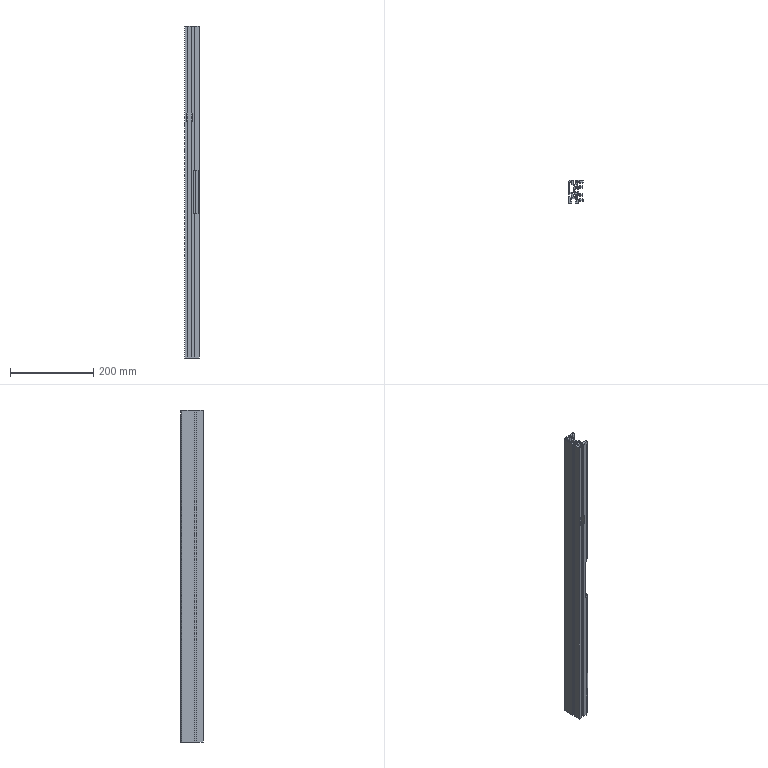Part | STEP file | Line rear chain guide rail L800 | 1 solid | 182 faces | box 35 x 55 x 800 mm | volume 614958 mm3 | plane 132 | cylinder 41 | cone 9 | commonest cylinder face diameters 2.5 x9 2 x8 6.5 x6 2.3 x4 11 x4 13 x4